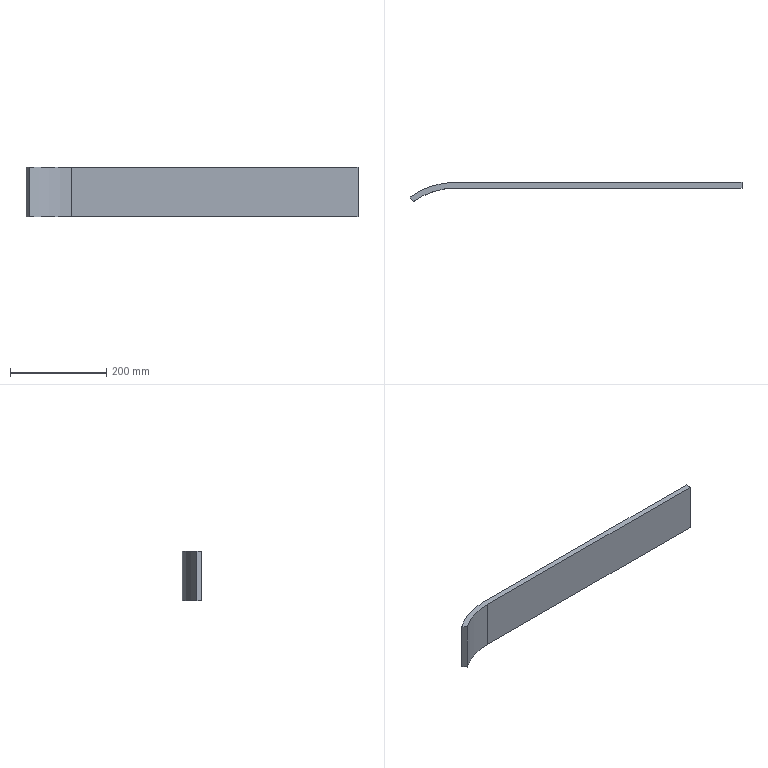Part | SolidWorks | features Extrusion 1 | 1 solid | 8 faces | box 690 x 40 x 102 mm | volume 847761 mm3 | plane 6 | cylinder 2 | commonest cylinder face diameters 300 x1 324 x1
STEP:
#1=CARTESIAN_POINT('',(0.,-12.,0.));
#2=VERTEX_POINT('',#1);
#3=CARTESIAN_POINT('',(0.,0.,0.));
#4=VERTEX_POINT('',#3);
#5=CARTESIAN_POINT('',(0.,0.,0.));
#6=DIRECTION('',(0.,1.,0.));
#7=VECTOR('',#6,1000.);
#8=LINE('',#5,#7);
#9=EDGE_CURVE('',#2,#4,#8,.T.);
#10=ORIENTED_EDGE('',*,*,#9,.T.);
#11=CARTESIAN_POINT('',(0.,0.,102.));
#12=VERTEX_POINT('',#11);
#13=CARTESIAN_POINT('',(0.,0.,102.));
#14=DIRECTION('',(0.,0.,-1.));
#15=VECTOR('',#14,1000.);
#16=LINE('',#13,#15);
#17=EDGE_CURVE('',#12,#4,#16,.T.);
#18=ORIENTED_EDGE('',*,*,#17,.F.);
#19=CARTESIAN_POINT('',(0.,-12.,102.));
#20=VERTEX_POINT('',#19);
#21=CARTESIAN_POINT('',(0.,0.,102.));
#22=DIRECTION('',(0.,1.,0.));
#23=VECTOR('',#22,1000.);
#24=LINE('',#21,#23);
#25=EDGE_CURVE('',#20,#12,#24,.T.);
#26=ORIENTED_EDGE('',*,*,#25,.F.);
#27=CARTESIAN_POINT('',(0.,-12.,102.));
#28=DIRECTION('',(0.,0.,-1.));
#29=VECTOR('',#28,1000.);
#30=LINE('',#27,#29);
#31=EDGE_CURVE('',#20,#2,#30,.T.);
#32=ORIENTED_EDGE('',*,*,#31,.T.);
#33=EDGE_LOOP('',(#10,#18,#26,#32));
#34=FACE_OUTER_BOUND('',#33,.T.);
#35=CARTESIAN_POINT('',(0.,0.,102.));
#36=DIRECTION('',(-1.,0.,0.));
#37=DIRECTION('',(0.,-1.,0.));
#38=AXIS2_PLACEMENT_3D('',#35,#36,#37);
#39=PLANE('',#38);
#40=ADVANCED_FACE('',(#34),#39,.F.);
#41=CARTESIAN_POINT('',(-595.749,0.,0.));
#42=VERTEX_POINT('',#41);
#43=CARTESIAN_POINT('',(0.,0.,0.));
#44=DIRECTION('',(-1.,0.,0.));
#45=VECTOR('',#44,1000.);
#46=LINE('',#43,#45);
#47=EDGE_CURVE('',#4,#42,#46,.T.);
#48=ORIENTED_EDGE('',*,*,#47,.T.);
#49=CARTESIAN_POINT('',(-595.749,0.,102.));
#50=VERTEX_POINT('',#49);
#51=CARTESIAN_POINT('',(-595.749,0.,102.));
#52=DIRECTION('',(0.,0.,-1.));
#53=VECTOR('',#52,1000.);
#54=LINE('',#51,#53);
#55=EDGE_CURVE('',#50,#42,#54,.T.);
#56=ORIENTED_EDGE('',*,*,#55,.F.);
#57=CARTESIAN_POINT('',(0.,0.,102.));
#58=DIRECTION('',(-1.,0.,0.));
#59=VECTOR('',#58,1000.);
#60=LINE('',#57,#59);
#61=EDGE_CURVE('',#12,#50,#60,.T.);
#62=ORIENTED_EDGE('',*,*,#61,.F.);
#63=ORIENTED_EDGE('',*,*,#17,.T.);
#64=EDGE_LOOP('',(#48,#56,#62,#63));
#65=FACE_OUTER_BOUND('',#64,.T.);
#66=CARTESIAN_POINT('',(0.,0.,102.));
#67=DIRECTION('',(0.,-1.,0.));
#68=DIRECTION('',(0.,0.,-1.));
#69=AXIS2_PLACEMENT_3D('',#66,#67,#68);
#70=PLANE('',#69);
#71=ADVANCED_FACE('',(#65),#70,.F.);
#72=CARTESIAN_POINT('',(-690.,-30.24,0.));
#73=VERTEX_POINT('',#72);
#74=CARTESIAN_POINT('',(-595.749,-162.,0.));
#75=DIRECTION('',(0.,0.,1.));
#76=DIRECTION('',(1.,0.,0.));
#77=AXIS2_PLACEMENT_3D('',#74,#75,#76);
#78=CIRCLE('',#77,162.);
#79=EDGE_CURVE('',#42,#73,#78,.T.);
#80=ORIENTED_EDGE('',*,*,#79,.T.);
#81=CARTESIAN_POINT('',(-690.,-30.24,102.));
#82=VERTEX_POINT('',#81);
#83=CARTESIAN_POINT('',(-690.,-30.24,102.));
#84=DIRECTION('',(0.,0.,-1.));
#85=VECTOR('',#84,1000.);
#86=LINE('',#83,#85);
#87=EDGE_CURVE('',#82,#73,#86,.T.);
#88=ORIENTED_EDGE('',*,*,#87,.F.);
#89=CARTESIAN_POINT('',(-595.749,-162.,102.));
#90=DIRECTION('',(0.,0.,1.));
#91=DIRECTION('',(1.,0.,0.));
#92=AXIS2_PLACEMENT_3D('',#89,#90,#91);
#93=CIRCLE('',#92,162.);
#94=EDGE_CURVE('',#50,#82,#93,.T.);
#95=ORIENTED_EDGE('',*,*,#94,.F.);
#96=ORIENTED_EDGE('',*,*,#55,.T.);
#97=EDGE_LOOP('',(#80,#88,#95,#96));
#98=FACE_OUTER_BOUND('',#97,.T.);
#99=CARTESIAN_POINT('',(-595.749,-162.,102.));
#100=DIRECTION('',(0.,0.,-1.));
#101=DIRECTION('',(-1.,0.,0.));
#102=AXIS2_PLACEMENT_3D('',#99,#100,#101);
#103=CYLINDRICAL_SURFACE('',#102,162.);
#104=ADVANCED_FACE('',(#98),#103,.T.);
#105=CARTESIAN_POINT('',(-683.018,-40.,0.));
#106=VERTEX_POINT('',#105);
#107=CARTESIAN_POINT('',(-683.018,-40.,0.));
#108=DIRECTION('',(0.5818,-0.8133,0.));
#109=VECTOR('',#108,1000.);
#110=LINE('',#107,#109);
#111=EDGE_CURVE('',#73,#106,#110,.T.);
#112=ORIENTED_EDGE('',*,*,#111,.T.);
#113=CARTESIAN_POINT('',(-683.018,-40.,102.));
#114=VERTEX_POINT('',#113);
#115=CARTESIAN_POINT('',(-683.018,-40.,102.));
#116=DIRECTION('',(0.,0.,-1.));
#117=VECTOR('',#116,1000.);
#118=LINE('',#115,#117);
#119=EDGE_CURVE('',#114,#106,#118,.T.);
#120=ORIENTED_EDGE('',*,*,#119,.F.);
#121=CARTESIAN_POINT('',(-683.018,-40.,102.));
#122=DIRECTION('',(0.5818,-0.8133,0.));
#123=VECTOR('',#122,1000.);
#124=LINE('',#121,#123);
#125=EDGE_CURVE('',#82,#114,#124,.T.);
#126=ORIENTED_EDGE('',*,*,#125,.F.);
#127=ORIENTED_EDGE('',*,*,#87,.T.);
#128=EDGE_LOOP('',(#112,#120,#126,#127));
#129=FACE_OUTER_BOUND('',#128,.T.);
#130=CARTESIAN_POINT('',(-683.018,-40.,102.));
#131=DIRECTION('',(0.8133,0.5818,0.));
#132=DIRECTION('',(-0.5818,0.8133,0.));
#133=AXIS2_PLACEMENT_3D('',#130,#131,#132);
#134=PLANE('',#133);
#135=ADVANCED_FACE('',(#129),#134,.F.);
#136=CARTESIAN_POINT('',(-595.749,-12.,0.));
#137=VERTEX_POINT('',#136);
#138=CARTESIAN_POINT('',(-595.749,-162.,0.));
#139=DIRECTION('',(0.,0.,-1.));
#140=DIRECTION('',(1.,0.,0.));
#141=AXIS2_PLACEMENT_3D('',#138,#139,#140);
#142=CIRCLE('',#141,150.);
#143=EDGE_CURVE('',#106,#137,#142,.T.);
#144=ORIENTED_EDGE('',*,*,#143,.T.);
#145=CARTESIAN_POINT('',(-595.749,-12.,102.));
#146=VERTEX_POINT('',#145);
#147=CARTESIAN_POINT('',(-595.749,-12.,102.));
#148=DIRECTION('',(0.,0.,-1.));
#149=VECTOR('',#148,1000.);
#150=LINE('',#147,#149);
#151=EDGE_CURVE('',#146,#137,#150,.T.);
#152=ORIENTED_EDGE('',*,*,#151,.F.);
#153=CARTESIAN_POINT('',(-595.749,-162.,102.));
#154=DIRECTION('',(0.,0.,-1.));
#155=DIRECTION('',(1.,0.,0.));
#156=AXIS2_PLACEMENT_3D('',#153,#154,#155);
#157=CIRCLE('',#156,150.);
#158=EDGE_CURVE('',#114,#146,#157,.T.);
#159=ORIENTED_EDGE('',*,*,#158,.F.);
#160=ORIENTED_EDGE('',*,*,#119,.T.);
#161=EDGE_LOOP('',(#144,#152,#159,#160));
#162=FACE_OUTER_BOUND('',#161,.T.);
#163=CARTESIAN_POINT('',(-595.749,-162.,102.));
#164=DIRECTION('',(0.,0.,-1.));
#165=DIRECTION('',(-1.,0.,0.));
#166=AXIS2_PLACEMENT_3D('',#163,#164,#165);
#167=CYLINDRICAL_SURFACE('',#166,150.);
#168=ADVANCED_FACE('',(#162),#167,.F.);
#169=CARTESIAN_POINT('',(0.,-12.,0.));
#170=DIRECTION('',(1.,0.,0.));
#171=VECTOR('',#170,1000.);
#172=LINE('',#169,#171);
#173=EDGE_CURVE('',#137,#2,#172,.T.);
#174=ORIENTED_EDGE('',*,*,#173,.T.);
#175=ORIENTED_EDGE('',*,*,#31,.F.);
#176=CARTESIAN_POINT('',(0.,-12.,102.));
#177=DIRECTION('',(1.,0.,0.));
#178=VECTOR('',#177,1000.);
#179=LINE('',#176,#178);
#180=EDGE_CURVE('',#146,#20,#179,.T.);
#181=ORIENTED_EDGE('',*,*,#180,.F.);
#182=ORIENTED_EDGE('',*,*,#151,.T.);
#183=EDGE_LOOP('',(#174,#175,#181,#182));
#184=FACE_OUTER_BOUND('',#183,.T.);
#185=CARTESIAN_POINT('',(0.,-12.,102.));
#186=DIRECTION('',(0.,1.,0.));
#187=DIRECTION('',(-1.,0.,0.));
#188=AXIS2_PLACEMENT_3D('',#185,#186,#187);
#189=PLANE('',#188);
#190=ADVANCED_FACE('',(#184),#189,.F.);
#191=ORIENTED_EDGE('',*,*,#25,.T.);
#192=ORIENTED_EDGE('',*,*,#61,.T.);
#193=ORIENTED_EDGE('',*,*,#94,.T.);
#194=ORIENTED_EDGE('',*,*,#125,.T.);
#195=ORIENTED_EDGE('',*,*,#158,.T.);
#196=ORIENTED_EDGE('',*,*,#180,.T.);
#197=EDGE_LOOP('',(#191,#192,#193,#194,#195,#196));
#198=FACE_OUTER_BOUND('',#197,.T.);
#199=CARTESIAN_POINT('',(-595.749,-162.,102.));
#200=DIRECTION('',(0.,0.,1.));
#201=DIRECTION('',(1.,0.,0.));
#202=AXIS2_PLACEMENT_3D('',#199,#200,#201);
#203=PLANE('',#202);
#204=ADVANCED_FACE('',(#198),#203,.T.);
#205=ORIENTED_EDGE('',*,*,#9,.F.);
#206=ORIENTED_EDGE('',*,*,#173,.F.);
#207=ORIENTED_EDGE('',*,*,#143,.F.);
#208=ORIENTED_EDGE('',*,*,#111,.F.);
#209=ORIENTED_EDGE('',*,*,#79,.F.);
#210=ORIENTED_EDGE('',*,*,#47,.F.);
#211=EDGE_LOOP('',(#205,#206,#207,#208,#209,#210));
#212=FACE_OUTER_BOUND('',#211,.T.);
#213=CARTESIAN_POINT('',(-595.749,-162.,0.));
#214=DIRECTION('',(0.,0.,1.));
#215=DIRECTION('',(1.,0.,0.));
#216=AXIS2_PLACEMENT_3D('',#213,#214,#215);
#217=PLANE('',#216);
#218=ADVANCED_FACE('',(#212),#217,.F.);
#219=CLOSED_SHELL('',(#40,#71,#104,#135,#168,#190,#204,#218));
#220=MANIFOLD_SOLID_BREP('',#219);
#221=CARTESIAN_POINT('',(0.,0.,0.));
#222=DIRECTION('',(0.,0.,1.));
#223=DIRECTION('',(1.,0.,0.));
#224=AXIS2_PLACEMENT_3D('',#221,#222,#223);
#225=(LENGTH_UNIT()NAMED_UNIT(*)SI_UNIT(.MILLI.,.METRE.));
#226=UNCERTAINTY_MEASURE_WITH_UNIT(LENGTH_MEASURE(0.00001),#225,'','');
#227=(NAMED_UNIT(*)PLANE_ANGLE_UNIT()SI_UNIT($,.RADIAN.));
#228=(NAMED_UNIT(*)SI_UNIT($,.STERADIAN.)SOLID_ANGLE_UNIT());
#229=(GEOMETRIC_REPRESENTATION_CONTEXT(3)GLOBAL_UNCERTAINTY_ASSIGNED_CONTEXT((#226))GLOBAL_UNIT_ASSIGNED_CONTEXT((#225,#227,#228))REPRESENTATION_CONTEXT('',''));
#230=ADVANCED_BREP_SHAPE_REPRESENTATION('',(#220,#224),#229);